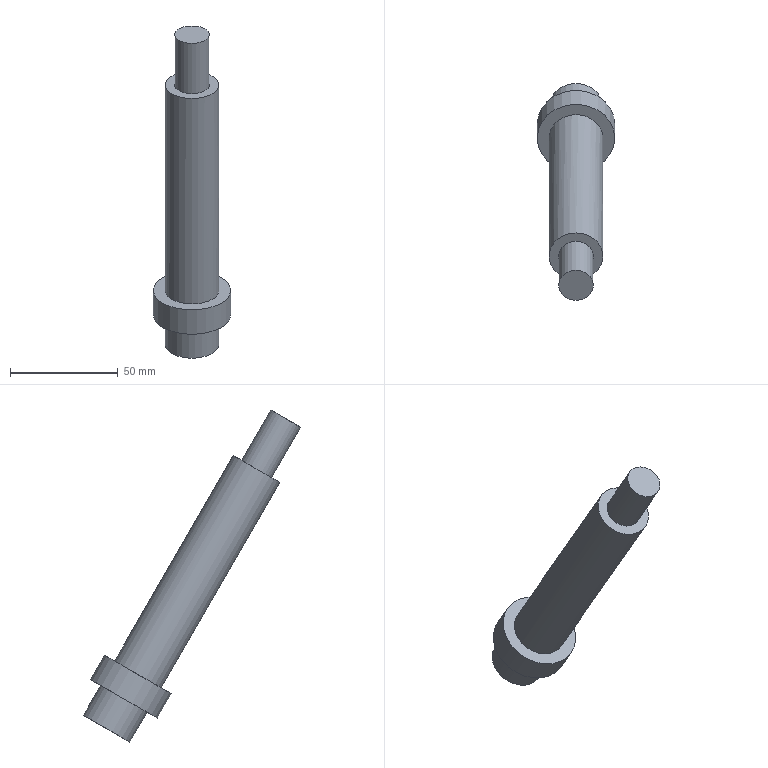Part | NX | features solid 2 | 1 solid | 9 faces | box 36 x 100.754 x 154.01 mm | volume 80511 mm3 | plane 5 | cylinder 4 | commonest cylinder face diameters 25 x2 16 x1 36 x1
STEP:
#1=CARTESIAN_POINT('',(385.,-498.723,99.923));
#2=VERTEX_POINT('',#1);
#3=CARTESIAN_POINT('',(385.,-491.795,103.923));
#4=DIRECTION('',(0.,0.5,-0.866));
#5=DIRECTION('',(0.,-0.866,-0.5));
#6=AXIS2_PLACEMENT_3D('',#3,#4,#5);
#7=CIRCLE('',#6,8.);
#8=EDGE_CURVE('',#2,#2,#7,.F.);
#9=ORIENTED_EDGE('',*,*,#8,.F.);
#10=EDGE_LOOP('',(#9));
#11=FACE_BOUND('',#10,.T.);
#12=CARTESIAN_POINT('',(385.,-502.62,97.673));
#13=VERTEX_POINT('',#12);
#14=CARTESIAN_POINT('',(385.,-491.795,103.923));
#15=DIRECTION('',(0.,0.5,-0.866));
#16=DIRECTION('',(0.,-0.866,-0.5));
#17=AXIS2_PLACEMENT_3D('',#14,#15,#16);
#18=CIRCLE('',#17,12.5);
#19=EDGE_CURVE('',#13,#13,#18,.T.);
#20=ORIENTED_EDGE('',*,*,#19,.F.);
#21=EDGE_LOOP('',(#20));
#22=FACE_BOUND('',#21,.T.);
#23=CARTESIAN_POINT('',(385.,-491.795,103.923));
#24=DIRECTION('',(0.,-0.5,0.866));
#25=DIRECTION('',(1.,0.,0.));
#26=AXIS2_PLACEMENT_3D('',#23,#24,#25);
#27=PLANE('',#26);
#28=ADVANCED_FACE('',(#11,#22),#27,.T.);
#29=CARTESIAN_POINT('',(397.5,-436.795,8.66));
#30=VERTEX_POINT('',#29);
#31=CARTESIAN_POINT('',(385.,-436.795,8.66));
#32=DIRECTION('',(0.,-0.5,0.866));
#33=DIRECTION('',(1.,0.,0.));
#34=AXIS2_PLACEMENT_3D('',#31,#32,#33);
#35=CIRCLE('',#34,12.5);
#36=EDGE_CURVE('',#30,#30,#35,.F.);
#37=ORIENTED_EDGE('',*,*,#36,.F.);
#38=EDGE_LOOP('',(#37));
#39=FACE_BOUND('',#38,.T.);
#40=ORIENTED_EDGE('',*,*,#19,.T.);
#41=EDGE_LOOP('',(#40));
#42=FACE_BOUND('',#41,.T.);
#43=CARTESIAN_POINT('',(385.,-556.795,216.506));
#44=DIRECTION('',(0.,0.5,-0.866));
#45=DIRECTION('',(-1.,0.,0.));
#46=AXIS2_PLACEMENT_3D('',#43,#44,#45);
#47=CYLINDRICAL_SURFACE('',#46,12.5);
#48=ADVANCED_FACE('',(#39,#42),#47,.T.);
#49=CARTESIAN_POINT('',(385.,-512.223,123.306));
#50=VERTEX_POINT('',#49);
#51=CARTESIAN_POINT('',(385.,-505.295,127.306));
#52=DIRECTION('',(0.,0.5,-0.866));
#53=DIRECTION('',(0.,-0.866,-0.5));
#54=AXIS2_PLACEMENT_3D('',#51,#52,#53);
#55=CIRCLE('',#54,8.);
#56=EDGE_CURVE('',#50,#50,#55,.T.);
#57=ORIENTED_EDGE('',*,*,#56,.F.);
#58=EDGE_LOOP('',(#57));
#59=FACE_BOUND('',#58,.T.);
#60=CARTESIAN_POINT('',(385.,-505.295,127.306));
#61=DIRECTION('',(0.,-0.5,0.866));
#62=DIRECTION('',(1.,0.,0.));
#63=AXIS2_PLACEMENT_3D('',#60,#61,#62);
#64=PLANE('',#63);
#65=ADVANCED_FACE('',(#59),#64,.T.);
#66=ORIENTED_EDGE('',*,*,#56,.T.);
#67=EDGE_LOOP('',(#66));
#68=FACE_BOUND('',#67,.T.);
#69=ORIENTED_EDGE('',*,*,#8,.T.);
#70=EDGE_LOOP('',(#69));
#71=FACE_BOUND('',#70,.T.);
#72=CARTESIAN_POINT('',(385.,-556.795,216.506));
#73=DIRECTION('',(0.,-0.5,0.866));
#74=DIRECTION('',(1.,0.,0.));
#75=AXIS2_PLACEMENT_3D('',#72,#73,#74);
#76=CYLINDRICAL_SURFACE('',#75,8.);
#77=ADVANCED_FACE('',(#68,#71),#76,.T.);
#78=CARTESIAN_POINT('',(372.5,-430.295,-2.598));
#79=VERTEX_POINT('',#78);
#80=CARTESIAN_POINT('',(385.,-430.295,-2.598));
#81=DIRECTION('',(0.,0.5,-0.866));
#82=DIRECTION('',(-1.,0.,0.));
#83=AXIS2_PLACEMENT_3D('',#80,#81,#82);
#84=CIRCLE('',#83,12.5);
#85=EDGE_CURVE('',#79,#79,#84,.T.);
#86=ORIENTED_EDGE('',*,*,#85,.F.);
#87=EDGE_LOOP('',(#86));
#88=FACE_BOUND('',#87,.T.);
#89=CARTESIAN_POINT('',(403.,-430.295,-2.598));
#90=VERTEX_POINT('',#89);
#91=CARTESIAN_POINT('',(385.,-430.295,-2.598));
#92=DIRECTION('',(0.,-0.5,0.866));
#93=DIRECTION('',(1.,0.,0.));
#94=AXIS2_PLACEMENT_3D('',#91,#92,#93);
#95=CIRCLE('',#94,18.);
#96=EDGE_CURVE('',#90,#90,#95,.T.);
#97=ORIENTED_EDGE('',*,*,#96,.F.);
#98=EDGE_LOOP('',(#97));
#99=FACE_BOUND('',#98,.T.);
#100=CARTESIAN_POINT('',(385.,-430.295,-2.598));
#101=DIRECTION('',(0.,0.5,-0.866));
#102=DIRECTION('',(-1.,0.,0.));
#103=AXIS2_PLACEMENT_3D('',#100,#101,#102);
#104=PLANE('',#103);
#105=ADVANCED_FACE('',(#88,#99),#104,.T.);
#106=ORIENTED_EDGE('',*,*,#36,.T.);
#107=EDGE_LOOP('',(#106));
#108=FACE_BOUND('',#107,.T.);
#109=CARTESIAN_POINT('',(367.,-436.795,8.66));
#110=VERTEX_POINT('',#109);
#111=CARTESIAN_POINT('',(385.,-436.795,8.66));
#112=DIRECTION('',(0.,0.5,-0.866));
#113=DIRECTION('',(-1.,0.,0.));
#114=AXIS2_PLACEMENT_3D('',#111,#112,#113);
#115=CIRCLE('',#114,18.);
#116=EDGE_CURVE('',#110,#110,#115,.T.);
#117=ORIENTED_EDGE('',*,*,#116,.F.);
#118=EDGE_LOOP('',(#117));
#119=FACE_BOUND('',#118,.T.);
#120=CARTESIAN_POINT('',(385.,-436.795,8.66));
#121=DIRECTION('',(0.,-0.5,0.866));
#122=DIRECTION('',(1.,0.,0.));
#123=AXIS2_PLACEMENT_3D('',#120,#121,#122);
#124=PLANE('',#123);
#125=ADVANCED_FACE('',(#108,#119),#124,.T.);
#126=ORIENTED_EDGE('',*,*,#96,.T.);
#127=EDGE_LOOP('',(#126));
#128=FACE_BOUND('',#127,.T.);
#129=ORIENTED_EDGE('',*,*,#116,.T.);
#130=EDGE_LOOP('',(#129));
#131=FACE_BOUND('',#130,.T.);
#132=CARTESIAN_POINT('',(385.,-436.795,8.66));
#133=DIRECTION('',(0.,0.5,-0.866));
#134=DIRECTION('',(-1.,0.,0.));
#135=AXIS2_PLACEMENT_3D('',#132,#133,#134);
#136=CYLINDRICAL_SURFACE('',#135,18.);
#137=ADVANCED_FACE('',(#128,#131),#136,.T.);
#138=CARTESIAN_POINT('',(397.5,-422.295,-16.454));
#139=VERTEX_POINT('',#138);
#140=CARTESIAN_POINT('',(385.,-422.295,-16.454));
#141=DIRECTION('',(0.,-0.5,0.866));
#142=DIRECTION('',(1.,0.,0.));
#143=AXIS2_PLACEMENT_3D('',#140,#141,#142);
#144=CIRCLE('',#143,12.5);
#145=EDGE_CURVE('',#139,#139,#144,.T.);
#146=ORIENTED_EDGE('',*,*,#145,.F.);
#147=EDGE_LOOP('',(#146));
#148=FACE_BOUND('',#147,.T.);
#149=CARTESIAN_POINT('',(385.,-422.295,-16.454));
#150=DIRECTION('',(0.,0.5,-0.866));
#151=DIRECTION('',(-1.,0.,0.));
#152=AXIS2_PLACEMENT_3D('',#149,#150,#151);
#153=PLANE('',#152);
#154=ADVANCED_FACE('',(#148),#153,.T.);
#155=ORIENTED_EDGE('',*,*,#145,.T.);
#156=EDGE_LOOP('',(#155));
#157=FACE_BOUND('',#156,.T.);
#158=ORIENTED_EDGE('',*,*,#85,.T.);
#159=EDGE_LOOP('',(#158));
#160=FACE_BOUND('',#159,.T.);
#161=CARTESIAN_POINT('',(385.,-430.295,-2.598));
#162=DIRECTION('',(0.,0.5,-0.866));
#163=DIRECTION('',(-1.,0.,0.));
#164=AXIS2_PLACEMENT_3D('',#161,#162,#163);
#165=CYLINDRICAL_SURFACE('',#164,12.5);
#166=ADVANCED_FACE('',(#157,#160),#165,.T.);
#167=CLOSED_SHELL('',(#28,#48,#65,#77,#105,#125,#137,#154,#166));
#168=MANIFOLD_SOLID_BREP('',#167);
#169=(LENGTH_UNIT()NAMED_UNIT(*)SI_UNIT(.MILLI.,.METRE.));
#170=UNCERTAINTY_MEASURE_WITH_UNIT(LENGTH_MEASURE(0.00001),#169,'','');
#171=(NAMED_UNIT(*)PLANE_ANGLE_UNIT()SI_UNIT($,.RADIAN.));
#172=(NAMED_UNIT(*)SI_UNIT($,.STERADIAN.)SOLID_ANGLE_UNIT());
#173=(GEOMETRIC_REPRESENTATION_CONTEXT(3)GLOBAL_UNCERTAINTY_ASSIGNED_CONTEXT((#170))GLOBAL_UNIT_ASSIGNED_CONTEXT((#169,#171,#172))REPRESENTATION_CONTEXT('',''));
#174=ADVANCED_BREP_SHAPE_REPRESENTATION('',(#168),#173);